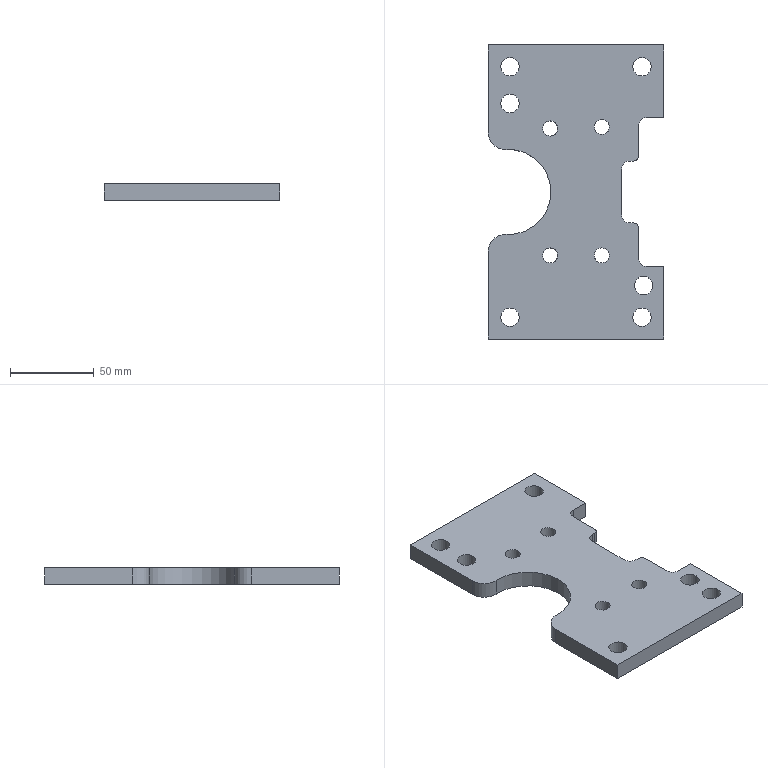Part | STEP file | PN_0047_id1022_x_t | 1 solid | 34 faces | box 105 x 176 x 10 mm | volume 142706 mm3 | cylinder 19 | plane 15 | commonest cylinder face diameters 11 x6 9 x4 10 x4 6 x2 20 x2 51 x1
STEP:
#1=CARTESIAN_POINT('',(213.,-88.,105.));
#2=VERTEX_POINT('',#1);
#3=CARTESIAN_POINT('',(213.,-35.444,105.));
#4=VERTEX_POINT('',#3);
#5=CARTESIAN_POINT('',(213.,-47.,105.));
#6=DIRECTION('',(0.,1.,0.));
#7=VECTOR('',#6,1.);
#8=LINE('',#5,#7);
#9=EDGE_CURVE('',#2,#4,#8,.T.);
#10=ORIENTED_EDGE('',*,*,#9,.T.);
#11=CARTESIAN_POINT('',(213.,-35.444,95.));
#12=VERTEX_POINT('',#11);
#13=CARTESIAN_POINT('',(213.,-35.444,95.));
#14=DIRECTION('',(0.,0.,-1.));
#15=VECTOR('',#14,1.);
#16=LINE('',#13,#15);
#17=EDGE_CURVE('',#4,#12,#16,.T.);
#18=ORIENTED_EDGE('',*,*,#17,.T.);
#19=CARTESIAN_POINT('',(213.,-88.,95.));
#20=VERTEX_POINT('',#19);
#21=CARTESIAN_POINT('',(213.,30.5,95.));
#22=DIRECTION('',(0.,1.,0.));
#23=VECTOR('',#22,1.);
#24=LINE('',#21,#23);
#25=EDGE_CURVE('',#20,#12,#24,.T.);
#26=ORIENTED_EDGE('',*,*,#25,.F.);
#27=CARTESIAN_POINT('',(213.,-88.,95.));
#28=DIRECTION('',(0.,0.,1.));
#29=VECTOR('',#28,1.);
#30=LINE('',#27,#29);
#31=EDGE_CURVE('',#20,#2,#30,.T.);
#32=ORIENTED_EDGE('',*,*,#31,.T.);
#33=EDGE_LOOP('',(#10,#18,#26,#32));
#34=FACE_OUTER_BOUND('',#33,.T.);
#35=CARTESIAN_POINT('',(213.,30.5,95.));
#36=DIRECTION('',(1.,0.,0.));
#37=DIRECTION('',(0.,1.,0.));
#38=AXIS2_PLACEMENT_3D('',#35,#36,#37);
#39=PLANE('',#38);
#40=ADVANCED_FACE('',(#34),#39,.F.);
#41=CARTESIAN_POINT('',(318.,88.,105.));
#42=VERTEX_POINT('',#41);
#43=CARTESIAN_POINT('',(318.,44.5,105.));
#44=VERTEX_POINT('',#43);
#45=CARTESIAN_POINT('',(318.,-47.,105.));
#46=DIRECTION('',(0.,-1.,0.));
#47=VECTOR('',#46,1.);
#48=LINE('',#45,#47);
#49=EDGE_CURVE('',#42,#44,#48,.T.);
#50=ORIENTED_EDGE('',*,*,#49,.T.);
#51=CARTESIAN_POINT('',(318.,44.5,95.));
#52=VERTEX_POINT('',#51);
#53=CARTESIAN_POINT('',(318.,44.5,95.));
#54=DIRECTION('',(0.,0.,-1.));
#55=VECTOR('',#54,1.);
#56=LINE('',#53,#55);
#57=EDGE_CURVE('',#44,#52,#56,.T.);
#58=ORIENTED_EDGE('',*,*,#57,.T.);
#59=CARTESIAN_POINT('',(318.,88.,95.));
#60=VERTEX_POINT('',#59);
#61=CARTESIAN_POINT('',(318.,30.5,95.));
#62=DIRECTION('',(0.,-1.,0.));
#63=VECTOR('',#62,1.);
#64=LINE('',#61,#63);
#65=EDGE_CURVE('',#60,#52,#64,.T.);
#66=ORIENTED_EDGE('',*,*,#65,.F.);
#67=CARTESIAN_POINT('',(318.,88.,95.));
#68=DIRECTION('',(0.,0.,1.));
#69=VECTOR('',#68,1.);
#70=LINE('',#67,#69);
#71=EDGE_CURVE('',#60,#42,#70,.T.);
#72=ORIENTED_EDGE('',*,*,#71,.T.);
#73=EDGE_LOOP('',(#50,#58,#66,#72));
#74=FACE_OUTER_BOUND('',#73,.T.);
#75=CARTESIAN_POINT('',(318.,30.5,95.));
#76=DIRECTION('',(-1.,0.,0.));
#77=DIRECTION('',(0.,-1.,0.));
#78=AXIS2_PLACEMENT_3D('',#75,#76,#77);
#79=PLANE('',#78);
#80=ADVANCED_FACE('',(#74),#79,.F.);
#81=CARTESIAN_POINT('',(318.,-44.5,105.));
#82=VERTEX_POINT('',#81);
#83=CARTESIAN_POINT('',(318.,-44.5,95.));
#84=VERTEX_POINT('',#83);
#85=CARTESIAN_POINT('',(318.,-44.5,95.));
#86=DIRECTION('',(0.,0.,-1.));
#87=VECTOR('',#86,1.);
#88=LINE('',#85,#87);
#89=EDGE_CURVE('',#82,#84,#88,.T.);
#90=ORIENTED_EDGE('',*,*,#89,.F.);
#91=CARTESIAN_POINT('',(318.,-88.,105.));
#92=VERTEX_POINT('',#91);
#93=CARTESIAN_POINT('',(318.,-47.,105.));
#94=DIRECTION('',(0.,-1.,0.));
#95=VECTOR('',#94,1.);
#96=LINE('',#93,#95);
#97=EDGE_CURVE('',#82,#92,#96,.T.);
#98=ORIENTED_EDGE('',*,*,#97,.T.);
#99=CARTESIAN_POINT('',(318.,-88.,95.));
#100=VERTEX_POINT('',#99);
#101=CARTESIAN_POINT('',(318.,-88.,95.));
#102=DIRECTION('',(0.,0.,1.));
#103=VECTOR('',#102,1.);
#104=LINE('',#101,#103);
#105=EDGE_CURVE('',#100,#92,#104,.T.);
#106=ORIENTED_EDGE('',*,*,#105,.F.);
#107=CARTESIAN_POINT('',(318.,30.5,95.));
#108=DIRECTION('',(0.,-1.,0.));
#109=VECTOR('',#108,1.);
#110=LINE('',#107,#109);
#111=EDGE_CURVE('',#84,#100,#110,.T.);
#112=ORIENTED_EDGE('',*,*,#111,.F.);
#113=EDGE_LOOP('',(#90,#98,#106,#112));
#114=FACE_OUTER_BOUND('',#113,.T.);
#115=CARTESIAN_POINT('',(318.,30.5,95.));
#116=DIRECTION('',(-1.,0.,0.));
#117=DIRECTION('',(0.,-1.,0.));
#118=AXIS2_PLACEMENT_3D('',#115,#116,#117);
#119=PLANE('',#118);
#120=ADVANCED_FACE('',(#114),#119,.F.);
#121=ORIENTED_EDGE('',*,*,#71,.F.);
#122=CARTESIAN_POINT('',(213.,88.,95.));
#123=VERTEX_POINT('',#122);
#124=CARTESIAN_POINT('',(265.5,88.,95.));
#125=DIRECTION('',(1.,0.,0.));
#126=VECTOR('',#125,1.);
#127=LINE('',#124,#126);
#128=EDGE_CURVE('',#123,#60,#127,.T.);
#129=ORIENTED_EDGE('',*,*,#128,.F.);
#130=CARTESIAN_POINT('',(213.,88.,105.));
#131=VERTEX_POINT('',#130);
#132=CARTESIAN_POINT('',(213.,88.,95.));
#133=DIRECTION('',(0.,0.,1.));
#134=VECTOR('',#133,1.);
#135=LINE('',#132,#134);
#136=EDGE_CURVE('',#123,#131,#135,.T.);
#137=ORIENTED_EDGE('',*,*,#136,.T.);
#138=CARTESIAN_POINT('',(-321.,88.,105.));
#139=DIRECTION('',(1.,0.,0.));
#140=VECTOR('',#139,1.);
#141=LINE('',#138,#140);
#142=EDGE_CURVE('',#131,#42,#141,.T.);
#143=ORIENTED_EDGE('',*,*,#142,.T.);
#144=EDGE_LOOP('',(#121,#129,#137,#143));
#145=FACE_OUTER_BOUND('',#144,.T.);
#146=CARTESIAN_POINT('',(265.5,88.,95.));
#147=DIRECTION('',(0.,-1.,0.));
#148=DIRECTION('',(1.,0.,0.));
#149=AXIS2_PLACEMENT_3D('',#146,#147,#148);
#150=PLANE('',#149);
#151=ADVANCED_FACE('',(#145),#150,.F.);
#152=CARTESIAN_POINT('',(213.,35.444,95.));
#153=VERTEX_POINT('',#152);
#154=CARTESIAN_POINT('',(213.,30.5,95.));
#155=DIRECTION('',(0.,1.,0.));
#156=VECTOR('',#155,1.);
#157=LINE('',#154,#156);
#158=EDGE_CURVE('',#153,#123,#157,.T.);
#159=ORIENTED_EDGE('',*,*,#158,.F.);
#160=CARTESIAN_POINT('',(213.,35.444,105.));
#161=VERTEX_POINT('',#160);
#162=CARTESIAN_POINT('',(213.,35.444,105.));
#163=DIRECTION('',(0.,0.,1.));
#164=VECTOR('',#163,1.);
#165=LINE('',#162,#164);
#166=EDGE_CURVE('',#153,#161,#165,.T.);
#167=ORIENTED_EDGE('',*,*,#166,.T.);
#168=CARTESIAN_POINT('',(213.,-47.,105.));
#169=DIRECTION('',(0.,1.,0.));
#170=VECTOR('',#169,1.);
#171=LINE('',#168,#170);
#172=EDGE_CURVE('',#161,#131,#171,.T.);
#173=ORIENTED_EDGE('',*,*,#172,.T.);
#174=ORIENTED_EDGE('',*,*,#136,.F.);
#175=EDGE_LOOP('',(#159,#167,#173,#174));
#176=FACE_OUTER_BOUND('',#175,.T.);
#177=CARTESIAN_POINT('',(213.,30.5,95.));
#178=DIRECTION('',(1.,0.,0.));
#179=DIRECTION('',(0.,1.,0.));
#180=AXIS2_PLACEMENT_3D('',#177,#178,#179);
#181=PLANE('',#180);
#182=ADVANCED_FACE('',(#176),#181,.F.);
#183=CARTESIAN_POINT('',(265.5,-88.,95.));
#184=DIRECTION('',(-1.,0.,0.));
#185=VECTOR('',#184,1.);
#186=LINE('',#183,#185);
#187=EDGE_CURVE('',#100,#20,#186,.T.);
#188=ORIENTED_EDGE('',*,*,#187,.F.);
#189=ORIENTED_EDGE('',*,*,#105,.T.);
#190=CARTESIAN_POINT('',(265.5,-88.,105.));
#191=DIRECTION('',(-1.,0.,0.));
#192=VECTOR('',#191,1.);
#193=LINE('',#190,#192);
#194=EDGE_CURVE('',#92,#2,#193,.T.);
#195=ORIENTED_EDGE('',*,*,#194,.T.);
#196=ORIENTED_EDGE('',*,*,#31,.F.);
#197=EDGE_LOOP('',(#188,#189,#195,#196));
#198=FACE_OUTER_BOUND('',#197,.T.);
#199=CARTESIAN_POINT('',(265.5,-88.,95.));
#200=DIRECTION('',(0.,-1.,0.));
#201=DIRECTION('',(0.,0.,1.));
#202=AXIS2_PLACEMENT_3D('',#199,#200,#201);
#203=PLANE('',#202);
#204=ADVANCED_FACE('',(#198),#203,.T.);
#205=CARTESIAN_POINT('',(300.5,-56.,105.));
#206=VERTEX_POINT('',#205);
#207=CARTESIAN_POINT('',(306.,-56.,105.));
#208=DIRECTION('',(0.,0.,-1.));
#209=DIRECTION('',(-1.,0.,0.));
#210=AXIS2_PLACEMENT_3D('',#207,#208,#209);
#211=CIRCLE('',#210,5.5);
#212=EDGE_CURVE('',#206,#206,#211,.T.);
#213=ORIENTED_EDGE('',*,*,#212,.T.);
#214=EDGE_LOOP('',(#213));
#215=FACE_BOUND('',#214,.T.);
#216=CARTESIAN_POINT('',(220.5,53.,105.));
#217=VERTEX_POINT('',#216);
#218=CARTESIAN_POINT('',(226.,53.,105.));
#219=DIRECTION('',(0.,0.,-1.));
#220=DIRECTION('',(-1.,0.,0.));
#221=AXIS2_PLACEMENT_3D('',#218,#219,#220);
#222=CIRCLE('',#221,5.5);
#223=EDGE_CURVE('',#217,#217,#222,.T.);
#224=ORIENTED_EDGE('',*,*,#223,.T.);
#225=EDGE_LOOP('',(#224));
#226=FACE_BOUND('',#225,.T.);
#227=CARTESIAN_POINT('',(220.5,-75.,105.));
#228=VERTEX_POINT('',#227);
#229=CARTESIAN_POINT('',(226.,-75.,105.));
#230=DIRECTION('',(0.,0.,1.));
#231=DIRECTION('',(-1.,0.,0.));
#232=AXIS2_PLACEMENT_3D('',#229,#230,#231);
#233=CIRCLE('',#232,5.5);
#234=EDGE_CURVE('',#228,#228,#233,.T.);
#235=ORIENTED_EDGE('',*,*,#234,.F.);
#236=EDGE_LOOP('',(#235));
#237=FACE_BOUND('',#236,.T.);
#238=CARTESIAN_POINT('',(310.5,-75.,105.));
#239=VERTEX_POINT('',#238);
#240=CARTESIAN_POINT('',(305.,-75.,105.));
#241=DIRECTION('',(0.,0.,-1.));
#242=DIRECTION('',(1.,0.,0.));
#243=AXIS2_PLACEMENT_3D('',#240,#241,#242);
#244=CIRCLE('',#243,5.5);
#245=EDGE_CURVE('',#239,#239,#244,.T.);
#246=ORIENTED_EDGE('',*,*,#245,.T.);
#247=EDGE_LOOP('',(#246));
#248=FACE_BOUND('',#247,.T.);
#249=CARTESIAN_POINT('',(220.5,75.,105.));
#250=VERTEX_POINT('',#249);
#251=CARTESIAN_POINT('',(226.,75.,105.));
#252=DIRECTION('',(0.,0.,-1.));
#253=DIRECTION('',(-1.,0.,0.));
#254=AXIS2_PLACEMENT_3D('',#251,#252,#253);
#255=CIRCLE('',#254,5.5);
#256=EDGE_CURVE('',#250,#250,#255,.T.);
#257=ORIENTED_EDGE('',*,*,#256,.T.);
#258=EDGE_LOOP('',(#257));
#259=FACE_BOUND('',#258,.T.);
#260=CARTESIAN_POINT('',(310.5,75.,105.));
#261=VERTEX_POINT('',#260);
#262=CARTESIAN_POINT('',(305.,75.,105.));
#263=DIRECTION('',(0.,0.,1.));
#264=DIRECTION('',(1.,0.,0.));
#265=AXIS2_PLACEMENT_3D('',#262,#263,#264);
#266=CIRCLE('',#265,5.5);
#267=EDGE_CURVE('',#261,#261,#266,.T.);
#268=ORIENTED_EDGE('',*,*,#267,.F.);
#269=EDGE_LOOP('',(#268));
#270=FACE_BOUND('',#269,.T.);
#271=CARTESIAN_POINT('',(250.,-42.5,105.));
#272=VERTEX_POINT('',#271);
#273=CARTESIAN_POINT('',(250.,-38.,105.));
#274=DIRECTION('',(0.,0.,1.));
#275=DIRECTION('',(0.,-1.,0.));
#276=AXIS2_PLACEMENT_3D('',#273,#274,#275);
#277=CIRCLE('',#276,4.5);
#278=EDGE_CURVE('',#272,#272,#277,.T.);
#279=ORIENTED_EDGE('',*,*,#278,.F.);
#280=EDGE_LOOP('',(#279));
#281=FACE_BOUND('',#280,.T.);
#282=CARTESIAN_POINT('',(281.,-33.5,105.));
#283=VERTEX_POINT('',#282);
#284=CARTESIAN_POINT('',(281.,-38.,105.));
#285=DIRECTION('',(0.,0.,1.));
#286=DIRECTION('',(0.,1.,0.));
#287=AXIS2_PLACEMENT_3D('',#284,#285,#286);
#288=CIRCLE('',#287,4.5);
#289=EDGE_CURVE('',#283,#283,#288,.T.);
#290=ORIENTED_EDGE('',*,*,#289,.F.);
#291=EDGE_LOOP('',(#290));
#292=FACE_BOUND('',#291,.T.);
#293=CARTESIAN_POINT('',(281.,34.5,105.));
#294=VERTEX_POINT('',#293);
#295=CARTESIAN_POINT('',(281.,39.,105.));
#296=DIRECTION('',(0.,0.,-1.));
#297=DIRECTION('',(0.,-1.,0.));
#298=AXIS2_PLACEMENT_3D('',#295,#296,#297);
#299=CIRCLE('',#298,4.5);
#300=EDGE_CURVE('',#294,#294,#299,.T.);
#301=ORIENTED_EDGE('',*,*,#300,.T.);
#302=EDGE_LOOP('',(#301));
#303=FACE_BOUND('',#302,.T.);
#304=CARTESIAN_POINT('',(250.,42.5,105.));
#305=VERTEX_POINT('',#304);
#306=CARTESIAN_POINT('',(250.,38.,105.));
#307=DIRECTION('',(0.,0.,-1.));
#308=DIRECTION('',(0.,1.,0.));
#309=AXIS2_PLACEMENT_3D('',#306,#307,#308);
#310=CIRCLE('',#309,4.5);
#311=EDGE_CURVE('',#305,#305,#310,.T.);
#312=ORIENTED_EDGE('',*,*,#311,.T.);
#313=EDGE_LOOP('',(#312));
#314=FACE_BOUND('',#313,.T.);
#315=ORIENTED_EDGE('',*,*,#172,.F.);
#316=CARTESIAN_POINT('',(223.563,25.459,105.));
#317=VERTEX_POINT('',#316);
#318=CARTESIAN_POINT('',(223.,35.444,105.));
#319=DIRECTION('',(0.,0.,1.));
#320=DIRECTION('',(1.,0.,0.));
#321=AXIS2_PLACEMENT_3D('',#318,#319,#320);
#322=CIRCLE('',#321,10.);
#323=EDGE_CURVE('',#161,#317,#322,.T.);
#324=ORIENTED_EDGE('',*,*,#323,.T.);
#325=CARTESIAN_POINT('',(223.563,-25.459,105.));
#326=VERTEX_POINT('',#325);
#327=CARTESIAN_POINT('',(225.,0.,105.));
#328=DIRECTION('',(0.,0.,1.));
#329=DIRECTION('',(1.,0.,0.));
#330=AXIS2_PLACEMENT_3D('',#327,#328,#329);
#331=CIRCLE('',#330,25.5);
#332=EDGE_CURVE('',#326,#317,#331,.T.);
#333=ORIENTED_EDGE('',*,*,#332,.F.);
#334=CARTESIAN_POINT('',(223.,-35.444,105.));
#335=DIRECTION('',(0.,0.,1.));
#336=DIRECTION('',(1.,0.,0.));
#337=AXIS2_PLACEMENT_3D('',#334,#335,#336);
#338=CIRCLE('',#337,10.);
#339=EDGE_CURVE('',#326,#4,#338,.T.);
#340=ORIENTED_EDGE('',*,*,#339,.T.);
#341=ORIENTED_EDGE('',*,*,#9,.F.);
#342=ORIENTED_EDGE('',*,*,#194,.F.);
#343=ORIENTED_EDGE('',*,*,#97,.F.);
#344=CARTESIAN_POINT('',(307.75,-44.5,105.));
#345=VERTEX_POINT('',#344);
#346=CARTESIAN_POINT('',(546.19,-44.5,105.));
#347=DIRECTION('',(-1.,0.,0.));
#348=VECTOR('',#347,1.);
#349=LINE('',#346,#348);
#350=EDGE_CURVE('',#82,#345,#349,.T.);
#351=ORIENTED_EDGE('',*,*,#350,.T.);
#352=CARTESIAN_POINT('',(302.75,-39.5,105.));
#353=VERTEX_POINT('',#352);
#354=CARTESIAN_POINT('',(307.75,-39.5,105.));
#355=DIRECTION('',(0.,0.,-1.));
#356=DIRECTION('',(1.,0.,0.));
#357=AXIS2_PLACEMENT_3D('',#354,#355,#356);
#358=CIRCLE('',#357,5.);
#359=EDGE_CURVE('',#345,#353,#358,.T.);
#360=ORIENTED_EDGE('',*,*,#359,.T.);
#361=CARTESIAN_POINT('',(302.75,-21.5,105.));
#362=VERTEX_POINT('',#361);
#363=CARTESIAN_POINT('',(302.75,-47.,105.));
#364=DIRECTION('',(0.,1.,0.));
#365=VECTOR('',#364,1.);
#366=LINE('',#363,#365);
#367=EDGE_CURVE('',#353,#362,#366,.T.);
#368=ORIENTED_EDGE('',*,*,#367,.T.);
#369=CARTESIAN_POINT('',(299.75,-18.5,105.));
#370=VERTEX_POINT('',#369);
#371=CARTESIAN_POINT('',(299.75,-21.5,105.));
#372=DIRECTION('',(0.,0.,1.));
#373=DIRECTION('',(1.,0.,0.));
#374=AXIS2_PLACEMENT_3D('',#371,#372,#373);
#375=CIRCLE('',#374,3.);
#376=EDGE_CURVE('',#362,#370,#375,.T.);
#377=ORIENTED_EDGE('',*,*,#376,.T.);
#378=CARTESIAN_POINT('',(297.75,-18.5,105.));
#379=VERTEX_POINT('',#378);
#380=CARTESIAN_POINT('',(-321.,-18.5,105.));
#381=DIRECTION('',(-1.,0.,0.));
#382=VECTOR('',#381,1.);
#383=LINE('',#380,#382);
#384=EDGE_CURVE('',#370,#379,#383,.T.);
#385=ORIENTED_EDGE('',*,*,#384,.T.);
#386=CARTESIAN_POINT('',(292.75,-13.5,105.));
#387=VERTEX_POINT('',#386);
#388=CARTESIAN_POINT('',(297.75,-13.5,105.));
#389=DIRECTION('',(0.,0.,-1.));
#390=DIRECTION('',(1.,0.,0.));
#391=AXIS2_PLACEMENT_3D('',#388,#389,#390);
#392=CIRCLE('',#391,5.);
#393=EDGE_CURVE('',#379,#387,#392,.T.);
#394=ORIENTED_EDGE('',*,*,#393,.T.);
#395=CARTESIAN_POINT('',(292.75,13.5,105.));
#396=VERTEX_POINT('',#395);
#397=CARTESIAN_POINT('',(292.75,-47.,105.));
#398=DIRECTION('',(0.,-1.,0.));
#399=VECTOR('',#398,1.);
#400=LINE('',#397,#399);
#401=EDGE_CURVE('',#396,#387,#400,.T.);
#402=ORIENTED_EDGE('',*,*,#401,.F.);
#403=CARTESIAN_POINT('',(297.75,18.5,105.));
#404=VERTEX_POINT('',#403);
#405=CARTESIAN_POINT('',(297.75,13.5,105.));
#406=DIRECTION('',(0.,0.,-1.));
#407=DIRECTION('',(1.,0.,0.));
#408=AXIS2_PLACEMENT_3D('',#405,#406,#407);
#409=CIRCLE('',#408,5.);
#410=EDGE_CURVE('',#396,#404,#409,.T.);
#411=ORIENTED_EDGE('',*,*,#410,.T.);
#412=CARTESIAN_POINT('',(299.75,18.5,105.));
#413=VERTEX_POINT('',#412);
#414=CARTESIAN_POINT('',(-321.,18.5,105.));
#415=DIRECTION('',(-1.,0.,0.));
#416=VECTOR('',#415,1.);
#417=LINE('',#414,#416);
#418=EDGE_CURVE('',#413,#404,#417,.T.);
#419=ORIENTED_EDGE('',*,*,#418,.F.);
#420=CARTESIAN_POINT('',(302.75,21.5,105.));
#421=VERTEX_POINT('',#420);
#422=CARTESIAN_POINT('',(299.75,21.5,105.));
#423=DIRECTION('',(0.,0.,-1.));
#424=DIRECTION('',(1.,0.,0.));
#425=AXIS2_PLACEMENT_3D('',#422,#423,#424);
#426=CIRCLE('',#425,3.);
#427=EDGE_CURVE('',#421,#413,#426,.T.);
#428=ORIENTED_EDGE('',*,*,#427,.F.);
#429=CARTESIAN_POINT('',(302.75,39.5,105.));
#430=VERTEX_POINT('',#429);
#431=CARTESIAN_POINT('',(302.75,-47.,105.));
#432=DIRECTION('',(0.,-1.,0.));
#433=VECTOR('',#432,1.);
#434=LINE('',#431,#433);
#435=EDGE_CURVE('',#430,#421,#434,.T.);
#436=ORIENTED_EDGE('',*,*,#435,.F.);
#437=CARTESIAN_POINT('',(307.75,44.5,105.));
#438=VERTEX_POINT('',#437);
#439=CARTESIAN_POINT('',(307.75,39.5,105.));
#440=DIRECTION('',(0.,0.,-1.));
#441=DIRECTION('',(1.,0.,0.));
#442=AXIS2_PLACEMENT_3D('',#439,#440,#441);
#443=CIRCLE('',#442,5.);
#444=EDGE_CURVE('',#430,#438,#443,.T.);
#445=ORIENTED_EDGE('',*,*,#444,.T.);
#446=CARTESIAN_POINT('',(266.,44.5,105.));
#447=DIRECTION('',(-1.,0.,0.));
#448=VECTOR('',#447,1.);
#449=LINE('',#446,#448);
#450=EDGE_CURVE('',#44,#438,#449,.T.);
#451=ORIENTED_EDGE('',*,*,#450,.F.);
#452=ORIENTED_EDGE('',*,*,#49,.F.);
#453=ORIENTED_EDGE('',*,*,#142,.F.);
#454=EDGE_LOOP('',(#315,#324,#333,#340,#341,#342,#343,#351,#360,#368,#377,#385,#394,#402,#411,#419,#428,#436,#445,#451,#452,#453));
#455=FACE_BOUND('',#454,.T.);
#456=CARTESIAN_POINT('',(-321.,-47.,105.));
#457=DIRECTION('',(0.,0.,1.));
#458=DIRECTION('',(1.,0.,0.));
#459=AXIS2_PLACEMENT_3D('',#456,#457,#458);
#460=PLANE('',#459);
#461=ADVANCED_FACE('',(#215,#226,#237,#248,#259,#270,#281,#292,#303,#314,#455),#460,.T.);
#462=CARTESIAN_POINT('',(300.5,-56.,95.));
#463=VERTEX_POINT('',#462);
#464=CARTESIAN_POINT('',(306.,-56.,95.));
#465=DIRECTION('',(0.,0.,1.));
#466=DIRECTION('',(-1.,0.,0.));
#467=AXIS2_PLACEMENT_3D('',#464,#465,#466);
#468=CIRCLE('',#467,5.5);
#469=EDGE_CURVE('',#463,#463,#468,.T.);
#470=ORIENTED_EDGE('',*,*,#469,.T.);
#471=EDGE_LOOP('',(#470));
#472=FACE_BOUND('',#471,.T.);
#473=CARTESIAN_POINT('',(220.5,53.,95.));
#474=VERTEX_POINT('',#473);
#475=CARTESIAN_POINT('',(226.,53.,95.));
#476=DIRECTION('',(0.,0.,1.));
#477=DIRECTION('',(-1.,0.,0.));
#478=AXIS2_PLACEMENT_3D('',#475,#476,#477);
#479=CIRCLE('',#478,5.5);
#480=EDGE_CURVE('',#474,#474,#479,.T.);
#481=ORIENTED_EDGE('',*,*,#480,.T.);
#482=EDGE_LOOP('',(#481));
#483=FACE_BOUND('',#482,.T.);
#484=CARTESIAN_POINT('',(231.5,-75.,95.));
#485=VERTEX_POINT('',#484);
#486=CARTESIAN_POINT('',(226.,-75.,95.));
#487=DIRECTION('',(0.,0.,1.));
#488=DIRECTION('',(1.,0.,0.));
#489=AXIS2_PLACEMENT_3D('',#486,#487,#488);
#490=CIRCLE('',#489,5.5);
#491=EDGE_CURVE('',#485,#485,#490,.T.);
#492=ORIENTED_EDGE('',*,*,#491,.T.);
#493=EDGE_LOOP('',(#492));
#494=FACE_BOUND('',#493,.T.);
#495=CARTESIAN_POINT('',(310.5,-75.,95.));
#496=VERTEX_POINT('',#495);
#497=CARTESIAN_POINT('',(305.,-75.,95.));
#498=DIRECTION('',(0.,0.,1.));
#499=DIRECTION('',(1.,0.,0.));
#500=AXIS2_PLACEMENT_3D('',#497,#498,#499);
#501=CIRCLE('',#500,5.5);
#502=EDGE_CURVE('',#496,#496,#501,.T.);
#503=ORIENTED_EDGE('',*,*,#502,.T.);
#504=EDGE_LOOP('',(#503));
#505=FACE_BOUND('',#504,.T.);
#506=CARTESIAN_POINT('',(231.5,75.,95.));
#507=VERTEX_POINT('',#506);
#508=CARTESIAN_POINT('',(226.,75.,95.));
#509=DIRECTION('',(0.,0.,1.));
#510=DIRECTION('',(1.,0.,0.));
#511=AXIS2_PLACEMENT_3D('',#508,#509,#510);
#512=CIRCLE('',#511,5.5);
#513=EDGE_CURVE('',#507,#507,#512,.T.);
#514=ORIENTED_EDGE('',*,*,#513,.T.);
#515=EDGE_LOOP('',(#514));
#516=FACE_BOUND('',#515,.T.);
#517=CARTESIAN_POINT('',(310.5,75.,95.));
#518=VERTEX_POINT('',#517);
#519=CARTESIAN_POINT('',(305.,75.,95.));
#520=DIRECTION('',(0.,0.,1.));
#521=DIRECTION('',(1.,0.,0.));
#522=AXIS2_PLACEMENT_3D('',#519,#520,#521);
#523=CIRCLE('',#522,5.5);
#524=EDGE_CURVE('',#518,#518,#523,.T.);
#525=ORIENTED_EDGE('',*,*,#524,.T.);
#526=EDGE_LOOP('',(#525));
#527=FACE_BOUND('',#526,.T.);
#528=CARTESIAN_POINT('',(254.5,-38.,95.));
#529=VERTEX_POINT('',#528);
#530=CARTESIAN_POINT('',(250.,-38.,95.));
#531=DIRECTION('',(0.,0.,1.));
#532=DIRECTION('',(1.,0.,0.));
#533=AXIS2_PLACEMENT_3D('',#530,#531,#532);
#534=CIRCLE('',#533,4.5);
#535=EDGE_CURVE('',#529,#529,#534,.T.);
#536=ORIENTED_EDGE('',*,*,#535,.T.);
#537=EDGE_LOOP('',(#536));
#538=FACE_BOUND('',#537,.T.);
#539=CARTESIAN_POINT('',(285.5,-38.,95.));
#540=VERTEX_POINT('',#539);
#541=CARTESIAN_POINT('',(281.,-38.,95.));
#542=DIRECTION('',(0.,0.,1.));
#543=DIRECTION('',(1.,0.,0.));
#544=AXIS2_PLACEMENT_3D('',#541,#542,#543);
#545=CIRCLE('',#544,4.5);
#546=EDGE_CURVE('',#540,#540,#545,.T.);
#547=ORIENTED_EDGE('',*,*,#546,.T.);
#548=EDGE_LOOP('',(#547));
#549=FACE_BOUND('',#548,.T.);
#550=CARTESIAN_POINT('',(285.5,39.,95.));
#551=VERTEX_POINT('',#550);
#552=CARTESIAN_POINT('',(281.,39.,95.));
#553=DIRECTION('',(0.,0.,1.));
#554=DIRECTION('',(1.,0.,0.));
#555=AXIS2_PLACEMENT_3D('',#552,#553,#554);
#556=CIRCLE('',#555,4.5);
#557=EDGE_CURVE('',#551,#551,#556,.T.);
#558=ORIENTED_EDGE('',*,*,#557,.T.);
#559=EDGE_LOOP('',(#558));
#560=FACE_BOUND('',#559,.T.);
#561=CARTESIAN_POINT('',(254.5,38.,95.));
#562=VERTEX_POINT('',#561);
#563=CARTESIAN_POINT('',(250.,38.,95.));
#564=DIRECTION('',(0.,0.,1.));
#565=DIRECTION('',(1.,0.,0.));
#566=AXIS2_PLACEMENT_3D('',#563,#564,#565);
#567=CIRCLE('',#566,4.5);
#568=EDGE_CURVE('',#562,#562,#567,.T.);
#569=ORIENTED_EDGE('',*,*,#568,.T.);
#570=EDGE_LOOP('',(#569));
#571=FACE_BOUND('',#570,.T.);
#572=CARTESIAN_POINT('',(223.563,-25.459,95.));
#573=VERTEX_POINT('',#572);
#574=CARTESIAN_POINT('',(223.563,25.459,95.));
#575=VERTEX_POINT('',#574);
#576=CARTESIAN_POINT('',(225.,0.,95.));
#577=DIRECTION('',(0.,0.,1.));
#578=DIRECTION('',(1.,0.,0.));
#579=AXIS2_PLACEMENT_3D('',#576,#577,#578);
#580=CIRCLE('',#579,25.5);
#581=EDGE_CURVE('',#573,#575,#580,.T.);
#582=ORIENTED_EDGE('',*,*,#581,.T.);
#583=CARTESIAN_POINT('',(223.,35.444,95.));
#584=DIRECTION('',(0.,0.,-1.));
#585=DIRECTION('',(1.,0.,0.));
#586=AXIS2_PLACEMENT_3D('',#583,#584,#585);
#587=CIRCLE('',#586,10.);
#588=EDGE_CURVE('',#575,#153,#587,.T.);
#589=ORIENTED_EDGE('',*,*,#588,.T.);
#590=ORIENTED_EDGE('',*,*,#158,.T.);
#591=ORIENTED_EDGE('',*,*,#128,.T.);
#592=ORIENTED_EDGE('',*,*,#65,.T.);
#593=CARTESIAN_POINT('',(307.75,44.5,95.));
#594=VERTEX_POINT('',#593);
#595=CARTESIAN_POINT('',(266.,44.5,95.));
#596=DIRECTION('',(-1.,0.,0.));
#597=VECTOR('',#596,1.);
#598=LINE('',#595,#597);
#599=EDGE_CURVE('',#52,#594,#598,.T.);
#600=ORIENTED_EDGE('',*,*,#599,.T.);
#601=CARTESIAN_POINT('',(302.75,39.5,95.));
#602=VERTEX_POINT('',#601);
#603=CARTESIAN_POINT('',(307.75,39.5,95.));
#604=DIRECTION('',(0.,0.,1.));
#605=DIRECTION('',(1.,0.,0.));
#606=AXIS2_PLACEMENT_3D('',#603,#604,#605);
#607=CIRCLE('',#606,5.);
#608=EDGE_CURVE('',#594,#602,#607,.T.);
#609=ORIENTED_EDGE('',*,*,#608,.T.);
#610=CARTESIAN_POINT('',(302.75,21.5,95.));
#611=VERTEX_POINT('',#610);
#612=CARTESIAN_POINT('',(302.75,52.5,95.));
#613=DIRECTION('',(0.,1.,0.));
#614=VECTOR('',#613,1.);
#615=LINE('',#612,#614);
#616=EDGE_CURVE('',#611,#602,#615,.T.);
#617=ORIENTED_EDGE('',*,*,#616,.F.);
#618=CARTESIAN_POINT('',(299.75,18.5,95.));
#619=VERTEX_POINT('',#618);
#620=CARTESIAN_POINT('',(299.75,21.5,95.));
#621=DIRECTION('',(0.,0.,1.));
#622=DIRECTION('',(1.,0.,0.));
#623=AXIS2_PLACEMENT_3D('',#620,#621,#622);
#624=CIRCLE('',#623,3.);
#625=EDGE_CURVE('',#619,#611,#624,.T.);
#626=ORIENTED_EDGE('',*,*,#625,.F.);
#627=CARTESIAN_POINT('',(297.75,18.5,95.));
#628=VERTEX_POINT('',#627);
#629=CARTESIAN_POINT('',(304.75,18.5,95.));
#630=DIRECTION('',(1.,0.,0.));
#631=VECTOR('',#630,1.);
#632=LINE('',#629,#631);
#633=EDGE_CURVE('',#628,#619,#632,.T.);
#634=ORIENTED_EDGE('',*,*,#633,.F.);
#635=CARTESIAN_POINT('',(292.75,13.5,95.));
#636=VERTEX_POINT('',#635);
#637=CARTESIAN_POINT('',(297.75,13.5,95.));
#638=DIRECTION('',(0.,0.,1.));
#639=DIRECTION('',(1.,0.,0.));
#640=AXIS2_PLACEMENT_3D('',#637,#638,#639);
#641=CIRCLE('',#640,5.);
#642=EDGE_CURVE('',#628,#636,#641,.T.);
#643=ORIENTED_EDGE('',*,*,#642,.T.);
#644=CARTESIAN_POINT('',(292.75,-13.5,95.));
#645=VERTEX_POINT('',#644);
#646=CARTESIAN_POINT('',(292.75,-47.,95.));
#647=DIRECTION('',(0.,-1.,0.));
#648=VECTOR('',#647,1.);
#649=LINE('',#646,#648);
#650=EDGE_CURVE('',#636,#645,#649,.T.);
#651=ORIENTED_EDGE('',*,*,#650,.T.);
#652=CARTESIAN_POINT('',(297.75,-18.5,95.));
#653=VERTEX_POINT('',#652);
#654=CARTESIAN_POINT('',(297.75,-13.5,95.));
#655=DIRECTION('',(0.,0.,1.));
#656=DIRECTION('',(1.,0.,0.));
#657=AXIS2_PLACEMENT_3D('',#654,#655,#656);
#658=CIRCLE('',#657,5.);
#659=EDGE_CURVE('',#645,#653,#658,.T.);
#660=ORIENTED_EDGE('',*,*,#659,.T.);
#661=CARTESIAN_POINT('',(299.75,-18.5,95.));
#662=VERTEX_POINT('',#661);
#663=CARTESIAN_POINT('',(304.75,-18.5,95.));
#664=DIRECTION('',(1.,0.,0.));
#665=VECTOR('',#664,1.);
#666=LINE('',#663,#665);
#667=EDGE_CURVE('',#653,#662,#666,.T.);
#668=ORIENTED_EDGE('',*,*,#667,.T.);
#669=CARTESIAN_POINT('',(302.75,-21.5,95.));
#670=VERTEX_POINT('',#669);
#671=CARTESIAN_POINT('',(299.75,-21.5,95.));
#672=DIRECTION('',(0.,0.,-1.));
#673=DIRECTION('',(1.,0.,0.));
#674=AXIS2_PLACEMENT_3D('',#671,#672,#673);
#675=CIRCLE('',#674,3.);
#676=EDGE_CURVE('',#662,#670,#675,.T.);
#677=ORIENTED_EDGE('',*,*,#676,.T.);
#678=CARTESIAN_POINT('',(302.75,-39.5,95.));
#679=VERTEX_POINT('',#678);
#680=CARTESIAN_POINT('',(302.75,-52.5,95.));
#681=DIRECTION('',(0.,-1.,0.));
#682=VECTOR('',#681,1.);
#683=LINE('',#680,#682);
#684=EDGE_CURVE('',#670,#679,#683,.T.);
#685=ORIENTED_EDGE('',*,*,#684,.T.);
#686=CARTESIAN_POINT('',(307.75,-44.5,95.));
#687=VERTEX_POINT('',#686);
#688=CARTESIAN_POINT('',(307.75,-39.5,95.));
#689=DIRECTION('',(0.,0.,1.));
#690=DIRECTION('',(1.,0.,0.));
#691=AXIS2_PLACEMENT_3D('',#688,#689,#690);
#692=CIRCLE('',#691,5.);
#693=EDGE_CURVE('',#679,#687,#692,.T.);
#694=ORIENTED_EDGE('',*,*,#693,.T.);
#695=CARTESIAN_POINT('',(546.19,-44.5,95.));
#696=DIRECTION('',(-1.,0.,0.));
#697=VECTOR('',#696,1.);
#698=LINE('',#695,#697);
#699=EDGE_CURVE('',#84,#687,#698,.T.);
#700=ORIENTED_EDGE('',*,*,#699,.F.);
#701=ORIENTED_EDGE('',*,*,#111,.T.);
#702=ORIENTED_EDGE('',*,*,#187,.T.);
#703=ORIENTED_EDGE('',*,*,#25,.T.);
#704=CARTESIAN_POINT('',(223.,-35.444,95.));
#705=DIRECTION('',(0.,0.,-1.));
#706=DIRECTION('',(1.,0.,0.));
#707=AXIS2_PLACEMENT_3D('',#704,#705,#706);
#708=CIRCLE('',#707,10.);
#709=EDGE_CURVE('',#12,#573,#708,.T.);
#710=ORIENTED_EDGE('',*,*,#709,.T.);
#711=EDGE_LOOP('',(#582,#589,#590,#591,#592,#600,#609,#617,#626,#634,#643,#651,#660,#668,#677,#685,#694,#700,#701,#702,#703,#710));
#712=FACE_BOUND('',#711,.T.);
#713=CARTESIAN_POINT('',(-321.,-47.,95.));
#714=DIRECTION('',(0.,0.,1.));
#715=DIRECTION('',(1.,0.,0.));
#716=AXIS2_PLACEMENT_3D('',#713,#714,#715);
#717=PLANE('',#716);
#718=ADVANCED_FACE('',(#472,#483,#494,#505,#516,#527,#538,#549,#560,#571,#712),#717,.F.);
#719=ORIENTED_EDGE('',*,*,#650,.F.);
#720=CARTESIAN_POINT('',(292.75,13.5,105.));
#721=DIRECTION('',(0.,0.,1.));
#722=VECTOR('',#721,1.);
#723=LINE('',#720,#722);
#724=EDGE_CURVE('',#636,#396,#723,.T.);
#725=ORIENTED_EDGE('',*,*,#724,.T.);
#726=ORIENTED_EDGE('',*,*,#401,.T.);
#727=CARTESIAN_POINT('',(292.75,-13.5,11.));
#728=DIRECTION('',(0.,0.,-1.));
#729=VECTOR('',#728,1.);
#730=LINE('',#727,#729);
#731=EDGE_CURVE('',#387,#645,#730,.T.);
#732=ORIENTED_EDGE('',*,*,#731,.T.);
#733=EDGE_LOOP('',(#719,#725,#726,#732));
#734=FACE_OUTER_BOUND('',#733,.T.);
#735=CARTESIAN_POINT('',(292.75,-13.,11.));
#736=DIRECTION('',(-1.,0.,0.));
#737=DIRECTION('',(0.,1.,0.));
#738=AXIS2_PLACEMENT_3D('',#735,#736,#737);
#739=PLANE('',#738);
#740=ADVANCED_FACE('',(#734),#739,.F.);
#741=ORIENTED_EDGE('',*,*,#699,.T.);
#742=CARTESIAN_POINT('',(307.75,-44.5,11.));
#743=DIRECTION('',(0.,0.,1.));
#744=VECTOR('',#743,1.);
#745=LINE('',#742,#744);
#746=EDGE_CURVE('',#687,#345,#745,.T.);
#747=ORIENTED_EDGE('',*,*,#746,.T.);
#748=ORIENTED_EDGE('',*,*,#350,.F.);
#749=ORIENTED_EDGE('',*,*,#89,.T.);
#750=EDGE_LOOP('',(#741,#747,#748,#749));
#751=FACE_OUTER_BOUND('',#750,.T.);
#752=CARTESIAN_POINT('',(546.19,-44.5,11.));
#753=DIRECTION('',(0.,-1.,0.));
#754=DIRECTION('',(-1.,0.,0.));
#755=AXIS2_PLACEMENT_3D('',#752,#753,#754);
#756=PLANE('',#755);
#757=ADVANCED_FACE('',(#751),#756,.F.);
#758=ORIENTED_EDGE('',*,*,#450,.T.);
#759=CARTESIAN_POINT('',(307.75,44.5,11.));
#760=DIRECTION('',(0.,0.,-1.));
#761=VECTOR('',#760,1.);
#762=LINE('',#759,#761);
#763=EDGE_CURVE('',#438,#594,#762,.T.);
#764=ORIENTED_EDGE('',*,*,#763,.T.);
#765=ORIENTED_EDGE('',*,*,#599,.F.);
#766=ORIENTED_EDGE('',*,*,#57,.F.);
#767=EDGE_LOOP('',(#758,#764,#765,#766));
#768=FACE_OUTER_BOUND('',#767,.T.);
#769=CARTESIAN_POINT('',(266.,44.5,11.));
#770=DIRECTION('',(0.,1.,0.));
#771=DIRECTION('',(1.,0.,0.));
#772=AXIS2_PLACEMENT_3D('',#769,#770,#771);
#773=PLANE('',#772);
#774=ADVANCED_FACE('',(#768),#773,.F.);
#775=ORIENTED_EDGE('',*,*,#418,.T.);
#776=CARTESIAN_POINT('',(297.75,18.5,95.));
#777=DIRECTION('',(0.,0.,-1.));
#778=VECTOR('',#777,1.);
#779=LINE('',#776,#778);
#780=EDGE_CURVE('',#404,#628,#779,.T.);
#781=ORIENTED_EDGE('',*,*,#780,.T.);
#782=ORIENTED_EDGE('',*,*,#633,.T.);
#783=CARTESIAN_POINT('',(299.75,18.5,44.));
#784=DIRECTION('',(0.,0.,-1.));
#785=VECTOR('',#784,1.);
#786=LINE('',#783,#785);
#787=EDGE_CURVE('',#413,#619,#786,.T.);
#788=ORIENTED_EDGE('',*,*,#787,.F.);
#789=EDGE_LOOP('',(#775,#781,#782,#788));
#790=FACE_OUTER_BOUND('',#789,.T.);
#791=CARTESIAN_POINT('',(304.75,18.5,44.));
#792=DIRECTION('',(0.,1.,0.));
#793=DIRECTION('',(0.,0.,1.));
#794=AXIS2_PLACEMENT_3D('',#791,#792,#793);
#795=PLANE('',#794);
#796=ADVANCED_FACE('',(#790),#795,.F.);
#797=ORIENTED_EDGE('',*,*,#427,.T.);
#798=ORIENTED_EDGE('',*,*,#787,.T.);
#799=ORIENTED_EDGE('',*,*,#625,.T.);
#800=CARTESIAN_POINT('',(302.75,21.5,44.));
#801=DIRECTION('',(0.,0.,-1.));
#802=VECTOR('',#801,1.);
#803=LINE('',#800,#802);
#804=EDGE_CURVE('',#421,#611,#803,.T.);
#805=ORIENTED_EDGE('',*,*,#804,.F.);
#806=EDGE_LOOP('',(#797,#798,#799,#805));
#807=FACE_OUTER_BOUND('',#806,.T.);
#808=CARTESIAN_POINT('',(299.75,21.5,44.));
#809=DIRECTION('',(0.,0.,1.));
#810=DIRECTION('',(1.,0.,0.));
#811=AXIS2_PLACEMENT_3D('',#808,#809,#810);
#812=CYLINDRICAL_SURFACE('',#811,3.);
#813=ADVANCED_FACE('',(#807),#812,.T.);
#814=ORIENTED_EDGE('',*,*,#616,.T.);
#815=CARTESIAN_POINT('',(302.75,39.5,44.));
#816=DIRECTION('',(0.,0.,1.));
#817=VECTOR('',#816,1.);
#818=LINE('',#815,#817);
#819=EDGE_CURVE('',#602,#430,#818,.T.);
#820=ORIENTED_EDGE('',*,*,#819,.T.);
#821=ORIENTED_EDGE('',*,*,#435,.T.);
#822=ORIENTED_EDGE('',*,*,#804,.T.);
#823=EDGE_LOOP('',(#814,#820,#821,#822));
#824=FACE_OUTER_BOUND('',#823,.T.);
#825=CARTESIAN_POINT('',(302.75,52.5,44.));
#826=DIRECTION('',(-1.,0.,0.));
#827=DIRECTION('',(0.,0.,1.));
#828=AXIS2_PLACEMENT_3D('',#825,#826,#827);
#829=PLANE('',#828);
#830=ADVANCED_FACE('',(#824),#829,.F.);
#831=ORIENTED_EDGE('',*,*,#667,.F.);
#832=CARTESIAN_POINT('',(297.75,-18.5,118.));
#833=DIRECTION('',(0.,0.,1.));
#834=VECTOR('',#833,1.);
#835=LINE('',#832,#834);
#836=EDGE_CURVE('',#653,#379,#835,.T.);
#837=ORIENTED_EDGE('',*,*,#836,.T.);
#838=ORIENTED_EDGE('',*,*,#384,.F.);
#839=CARTESIAN_POINT('',(299.75,-18.5,118.));
#840=DIRECTION('',(0.,0.,-1.));
#841=VECTOR('',#840,1.);
#842=LINE('',#839,#841);
#843=EDGE_CURVE('',#370,#662,#842,.T.);
#844=ORIENTED_EDGE('',*,*,#843,.T.);
#845=EDGE_LOOP('',(#831,#837,#838,#844));
#846=FACE_OUTER_BOUND('',#845,.T.);
#847=CARTESIAN_POINT('',(304.75,-18.5,118.));
#848=DIRECTION('',(0.,1.,0.));
#849=DIRECTION('',(0.,0.,-1.));
#850=AXIS2_PLACEMENT_3D('',#847,#848,#849);
#851=PLANE('',#850);
#852=ADVANCED_FACE('',(#846),#851,.T.);
#853=ORIENTED_EDGE('',*,*,#376,.F.);
#854=CARTESIAN_POINT('',(302.75,-21.5,118.));
#855=DIRECTION('',(0.,0.,-1.));
#856=VECTOR('',#855,1.);
#857=LINE('',#854,#856);
#858=EDGE_CURVE('',#362,#670,#857,.T.);
#859=ORIENTED_EDGE('',*,*,#858,.T.);
#860=ORIENTED_EDGE('',*,*,#676,.F.);
#861=ORIENTED_EDGE('',*,*,#843,.F.);
#862=EDGE_LOOP('',(#853,#859,#860,#861));
#863=FACE_OUTER_BOUND('',#862,.T.);
#864=CARTESIAN_POINT('',(299.75,-21.5,118.));
#865=DIRECTION('',(0.,0.,-1.));
#866=DIRECTION('',(-1.,0.,0.));
#867=AXIS2_PLACEMENT_3D('',#864,#865,#866);
#868=CYLINDRICAL_SURFACE('',#867,3.);
#869=ADVANCED_FACE('',(#863),#868,.T.);
#870=ORIENTED_EDGE('',*,*,#367,.F.);
#871=CARTESIAN_POINT('',(302.75,-39.5,118.));
#872=DIRECTION('',(0.,0.,-1.));
#873=VECTOR('',#872,1.);
#874=LINE('',#871,#873);
#875=EDGE_CURVE('',#353,#679,#874,.T.);
#876=ORIENTED_EDGE('',*,*,#875,.T.);
#877=ORIENTED_EDGE('',*,*,#684,.F.);
#878=ORIENTED_EDGE('',*,*,#858,.F.);
#879=EDGE_LOOP('',(#870,#876,#877,#878));
#880=FACE_OUTER_BOUND('',#879,.T.);
#881=CARTESIAN_POINT('',(302.75,-52.5,118.));
#882=DIRECTION('',(1.,0.,0.));
#883=DIRECTION('',(0.,0.,-1.));
#884=AXIS2_PLACEMENT_3D('',#881,#882,#883);
#885=PLANE('',#884);
#886=ADVANCED_FACE('',(#880),#885,.T.);
#887=ORIENTED_EDGE('',*,*,#608,.F.);
#888=ORIENTED_EDGE('',*,*,#763,.F.);
#889=ORIENTED_EDGE('',*,*,#444,.F.);
#890=ORIENTED_EDGE('',*,*,#819,.F.);
#891=EDGE_LOOP('',(#887,#888,#889,#890));
#892=FACE_OUTER_BOUND('',#891,.T.);
#893=CARTESIAN_POINT('',(307.75,39.5,44.));
#894=DIRECTION('',(0.,0.,-1.));
#895=DIRECTION('',(-1.,0.,0.));
#896=AXIS2_PLACEMENT_3D('',#893,#894,#895);
#897=CYLINDRICAL_SURFACE('',#896,5.);
#898=ADVANCED_FACE('',(#892),#897,.F.);
#899=ORIENTED_EDGE('',*,*,#410,.F.);
#900=ORIENTED_EDGE('',*,*,#724,.F.);
#901=ORIENTED_EDGE('',*,*,#642,.F.);
#902=ORIENTED_EDGE('',*,*,#780,.F.);
#903=EDGE_LOOP('',(#899,#900,#901,#902));
#904=FACE_OUTER_BOUND('',#903,.T.);
#905=CARTESIAN_POINT('',(297.75,13.5,44.));
#906=DIRECTION('',(0.,0.,1.));
#907=DIRECTION('',(1.,0.,0.));
#908=AXIS2_PLACEMENT_3D('',#905,#906,#907);
#909=CYLINDRICAL_SURFACE('',#908,5.);
#910=ADVANCED_FACE('',(#904),#909,.F.);
#911=ORIENTED_EDGE('',*,*,#693,.F.);
#912=ORIENTED_EDGE('',*,*,#875,.F.);
#913=ORIENTED_EDGE('',*,*,#359,.F.);
#914=ORIENTED_EDGE('',*,*,#746,.F.);
#915=EDGE_LOOP('',(#911,#912,#913,#914));
#916=FACE_OUTER_BOUND('',#915,.T.);
#917=CARTESIAN_POINT('',(307.75,-39.5,11.));
#918=DIRECTION('',(0.,0.,1.));
#919=DIRECTION('',(1.,0.,0.));
#920=AXIS2_PLACEMENT_3D('',#917,#918,#919);
#921=CYLINDRICAL_SURFACE('',#920,5.);
#922=ADVANCED_FACE('',(#916),#921,.F.);
#923=ORIENTED_EDGE('',*,*,#393,.F.);
#924=ORIENTED_EDGE('',*,*,#836,.F.);
#925=ORIENTED_EDGE('',*,*,#659,.F.);
#926=ORIENTED_EDGE('',*,*,#731,.F.);
#927=EDGE_LOOP('',(#923,#924,#925,#926));
#928=FACE_OUTER_BOUND('',#927,.T.);
#929=CARTESIAN_POINT('',(297.75,-13.5,11.));
#930=DIRECTION('',(0.,0.,-1.));
#931=DIRECTION('',(-1.,0.,0.));
#932=AXIS2_PLACEMENT_3D('',#929,#930,#931);
#933=CYLINDRICAL_SURFACE('',#932,5.);
#934=ADVANCED_FACE('',(#928),#933,.F.);
#935=ORIENTED_EDGE('',*,*,#332,.T.);
#936=CARTESIAN_POINT('',(223.563,25.459,71.));
#937=DIRECTION('',(0.,0.,-1.));
#938=VECTOR('',#937,1.);
#939=LINE('',#936,#938);
#940=EDGE_CURVE('',#317,#575,#939,.T.);
#941=ORIENTED_EDGE('',*,*,#940,.T.);
#942=ORIENTED_EDGE('',*,*,#581,.F.);
#943=CARTESIAN_POINT('',(223.563,-25.459,71.));
#944=DIRECTION('',(0.,0.,1.));
#945=VECTOR('',#944,1.);
#946=LINE('',#943,#945);
#947=EDGE_CURVE('',#573,#326,#946,.T.);
#948=ORIENTED_EDGE('',*,*,#947,.T.);
#949=EDGE_LOOP('',(#935,#941,#942,#948));
#950=FACE_OUTER_BOUND('',#949,.T.);
#951=CARTESIAN_POINT('',(225.,0.,71.));
#952=DIRECTION('',(0.,0.,-1.));
#953=DIRECTION('',(0.,1.,0.));
#954=AXIS2_PLACEMENT_3D('',#951,#952,#953);
#955=CYLINDRICAL_SURFACE('',#954,25.5);
#956=ADVANCED_FACE('',(#950),#955,.F.);
#957=ORIENTED_EDGE('',*,*,#323,.F.);
#958=ORIENTED_EDGE('',*,*,#166,.F.);
#959=ORIENTED_EDGE('',*,*,#588,.F.);
#960=ORIENTED_EDGE('',*,*,#940,.F.);
#961=EDGE_LOOP('',(#957,#958,#959,#960));
#962=FACE_OUTER_BOUND('',#961,.T.);
#963=CARTESIAN_POINT('',(223.,35.444,71.));
#964=DIRECTION('',(0.,0.,-1.));
#965=DIRECTION('',(0.,1.,0.));
#966=AXIS2_PLACEMENT_3D('',#963,#964,#965);
#967=CYLINDRICAL_SURFACE('',#966,10.);
#968=ADVANCED_FACE('',(#962),#967,.T.);
#969=ORIENTED_EDGE('',*,*,#709,.F.);
#970=ORIENTED_EDGE('',*,*,#17,.F.);
#971=ORIENTED_EDGE('',*,*,#339,.F.);
#972=ORIENTED_EDGE('',*,*,#947,.F.);
#973=EDGE_LOOP('',(#969,#970,#971,#972));
#974=FACE_OUTER_BOUND('',#973,.T.);
#975=CARTESIAN_POINT('',(223.,-35.444,71.));
#976=DIRECTION('',(0.,0.,-1.));
#977=DIRECTION('',(0.,1.,0.));
#978=AXIS2_PLACEMENT_3D('',#975,#976,#977);
#979=CYLINDRICAL_SURFACE('',#978,10.);
#980=ADVANCED_FACE('',(#974),#979,.T.);
#981=ORIENTED_EDGE('',*,*,#311,.F.);
#982=EDGE_LOOP('',(#981));
#983=FACE_BOUND('',#982,.T.);
#984=ORIENTED_EDGE('',*,*,#568,.F.);
#985=EDGE_LOOP('',(#984));
#986=FACE_BOUND('',#985,.T.);
#987=CARTESIAN_POINT('',(250.,38.,105.));
#988=DIRECTION('',(0.,0.,-1.));
#989=DIRECTION('',(0.,1.,0.));
#990=AXIS2_PLACEMENT_3D('',#987,#988,#989);
#991=CYLINDRICAL_SURFACE('',#990,4.5);
#992=ADVANCED_FACE('',(#983,#986),#991,.F.);
#993=ORIENTED_EDGE('',*,*,#300,.F.);
#994=EDGE_LOOP('',(#993));
#995=FACE_BOUND('',#994,.T.);
#996=ORIENTED_EDGE('',*,*,#557,.F.);
#997=EDGE_LOOP('',(#996));
#998=FACE_BOUND('',#997,.T.);
#999=CARTESIAN_POINT('',(281.,39.,105.));
#1000=DIRECTION('',(0.,0.,-1.));
#1001=DIRECTION('',(0.,-1.,0.));
#1002=AXIS2_PLACEMENT_3D('',#999,#1000,#1001);
#1003=CYLINDRICAL_SURFACE('',#1002,4.5);
#1004=ADVANCED_FACE('',(#995,#998),#1003,.F.);
#1005=ORIENTED_EDGE('',*,*,#289,.T.);
#1006=EDGE_LOOP('',(#1005));
#1007=FACE_BOUND('',#1006,.T.);
#1008=ORIENTED_EDGE('',*,*,#546,.F.);
#1009=EDGE_LOOP('',(#1008));
#1010=FACE_BOUND('',#1009,.T.);
#1011=CARTESIAN_POINT('',(281.,-38.,105.));
#1012=DIRECTION('',(0.,0.,-1.));
#1013=DIRECTION('',(0.,1.,0.));
#1014=AXIS2_PLACEMENT_3D('',#1011,#1012,#1013);
#1015=CYLINDRICAL_SURFACE('',#1014,4.5);
#1016=ADVANCED_FACE('',(#1007,#1010),#1015,.F.);
#1017=ORIENTED_EDGE('',*,*,#278,.T.);
#1018=EDGE_LOOP('',(#1017));
#1019=FACE_BOUND('',#1018,.T.);
#1020=ORIENTED_EDGE('',*,*,#535,.F.);
#1021=EDGE_LOOP('',(#1020));
#1022=FACE_BOUND('',#1021,.T.);
#1023=CARTESIAN_POINT('',(250.,-38.,105.));
#1024=DIRECTION('',(0.,0.,-1.));
#1025=DIRECTION('',(0.,-1.,0.));
#1026=AXIS2_PLACEMENT_3D('',#1023,#1024,#1025);
#1027=CYLINDRICAL_SURFACE('',#1026,4.5);
#1028=ADVANCED_FACE('',(#1019,#1022),#1027,.F.);
#1029=ORIENTED_EDGE('',*,*,#267,.T.);
#1030=EDGE_LOOP('',(#1029));
#1031=FACE_BOUND('',#1030,.T.);
#1032=ORIENTED_EDGE('',*,*,#524,.F.);
#1033=EDGE_LOOP('',(#1032));
#1034=FACE_BOUND('',#1033,.T.);
#1035=CARTESIAN_POINT('',(305.,75.,105.));
#1036=DIRECTION('',(0.,0.,-1.));
#1037=DIRECTION('',(1.,0.,0.));
#1038=AXIS2_PLACEMENT_3D('',#1035,#1036,#1037);
#1039=CYLINDRICAL_SURFACE('',#1038,5.5);
#1040=ADVANCED_FACE('',(#1031,#1034),#1039,.F.);
#1041=ORIENTED_EDGE('',*,*,#256,.F.);
#1042=EDGE_LOOP('',(#1041));
#1043=FACE_BOUND('',#1042,.T.);
#1044=ORIENTED_EDGE('',*,*,#513,.F.);
#1045=EDGE_LOOP('',(#1044));
#1046=FACE_BOUND('',#1045,.T.);
#1047=CARTESIAN_POINT('',(226.,75.,105.));
#1048=DIRECTION('',(0.,0.,-1.));
#1049=DIRECTION('',(-1.,0.,0.));
#1050=AXIS2_PLACEMENT_3D('',#1047,#1048,#1049);
#1051=CYLINDRICAL_SURFACE('',#1050,5.5);
#1052=ADVANCED_FACE('',(#1043,#1046),#1051,.F.);
#1053=ORIENTED_EDGE('',*,*,#245,.F.);
#1054=EDGE_LOOP('',(#1053));
#1055=FACE_BOUND('',#1054,.T.);
#1056=ORIENTED_EDGE('',*,*,#502,.F.);
#1057=EDGE_LOOP('',(#1056));
#1058=FACE_BOUND('',#1057,.T.);
#1059=CARTESIAN_POINT('',(305.,-75.,105.));
#1060=DIRECTION('',(0.,0.,-1.));
#1061=DIRECTION('',(1.,0.,0.));
#1062=AXIS2_PLACEMENT_3D('',#1059,#1060,#1061);
#1063=CYLINDRICAL_SURFACE('',#1062,5.5);
#1064=ADVANCED_FACE('',(#1055,#1058),#1063,.F.);
#1065=ORIENTED_EDGE('',*,*,#234,.T.);
#1066=EDGE_LOOP('',(#1065));
#1067=FACE_BOUND('',#1066,.T.);
#1068=ORIENTED_EDGE('',*,*,#491,.F.);
#1069=EDGE_LOOP('',(#1068));
#1070=FACE_BOUND('',#1069,.T.);
#1071=CARTESIAN_POINT('',(226.,-75.,105.));
#1072=DIRECTION('',(0.,0.,-1.));
#1073=DIRECTION('',(-1.,0.,0.));
#1074=AXIS2_PLACEMENT_3D('',#1071,#1072,#1073);
#1075=CYLINDRICAL_SURFACE('',#1074,5.5);
#1076=ADVANCED_FACE('',(#1067,#1070),#1075,.F.);
#1077=ORIENTED_EDGE('',*,*,#480,.F.);
#1078=EDGE_LOOP('',(#1077));
#1079=FACE_BOUND('',#1078,.T.);
#1080=ORIENTED_EDGE('',*,*,#223,.F.);
#1081=EDGE_LOOP('',(#1080));
#1082=FACE_BOUND('',#1081,.T.);
#1083=CARTESIAN_POINT('',(226.,53.,105.));
#1084=DIRECTION('',(0.,0.,-1.));
#1085=DIRECTION('',(-1.,0.,0.));
#1086=AXIS2_PLACEMENT_3D('',#1083,#1084,#1085);
#1087=CYLINDRICAL_SURFACE('',#1086,5.5);
#1088=ADVANCED_FACE('',(#1079,#1082),#1087,.F.);
#1089=ORIENTED_EDGE('',*,*,#469,.F.);
#1090=EDGE_LOOP('',(#1089));
#1091=FACE_BOUND('',#1090,.T.);
#1092=ORIENTED_EDGE('',*,*,#212,.F.);
#1093=EDGE_LOOP('',(#1092));
#1094=FACE_BOUND('',#1093,.T.);
#1095=CARTESIAN_POINT('',(306.,-56.,105.));
#1096=DIRECTION('',(0.,0.,-1.));
#1097=DIRECTION('',(-1.,0.,0.));
#1098=AXIS2_PLACEMENT_3D('',#1095,#1096,#1097);
#1099=CYLINDRICAL_SURFACE('',#1098,5.5);
#1100=ADVANCED_FACE('',(#1091,#1094),#1099,.F.);
#1101=CLOSED_SHELL('',(#40,#80,#120,#151,#182,#204,#461,#718,#740,#757,#774,#796,#813,#830,#852,#869,#886,#898,#910,#922,#934,#956,#968,#980,#992,#1004,#1016,#1028,#1040,#1052,#1064,#1076,#1088,#1100));
#1102=MANIFOLD_SOLID_BREP('',#1101);
#1103=(LENGTH_UNIT()NAMED_UNIT(*)SI_UNIT(.MILLI.,.METRE.));
#1104=UNCERTAINTY_MEASURE_WITH_UNIT(LENGTH_MEASURE(0.00002),#1103,'','');
#1105=(NAMED_UNIT(*)PLANE_ANGLE_UNIT()SI_UNIT($,.RADIAN.));
#1106=PLANE_ANGLE_MEASURE_WITH_UNIT(PLANE_ANGLE_MEASURE(0.01745),#1105);
#1107=DIMENSIONAL_EXPONENTS(0.,0.,0.,0.,0.,0.,0.);
#1108=(CONVERSION_BASED_UNIT('DEGREE',#1106)NAMED_UNIT(#1107)PLANE_ANGLE_UNIT());
#1109=(NAMED_UNIT(*)SI_UNIT($,.STERADIAN.)SOLID_ANGLE_UNIT());
#1110=(GEOMETRIC_REPRESENTATION_CONTEXT(3)GLOBAL_UNCERTAINTY_ASSIGNED_CONTEXT((#1104))GLOBAL_UNIT_ASSIGNED_CONTEXT((#1103,#1108,#1109))REPRESENTATION_CONTEXT('',''));
#1111=ADVANCED_BREP_SHAPE_REPRESENTATION('',(#1102),#1110);